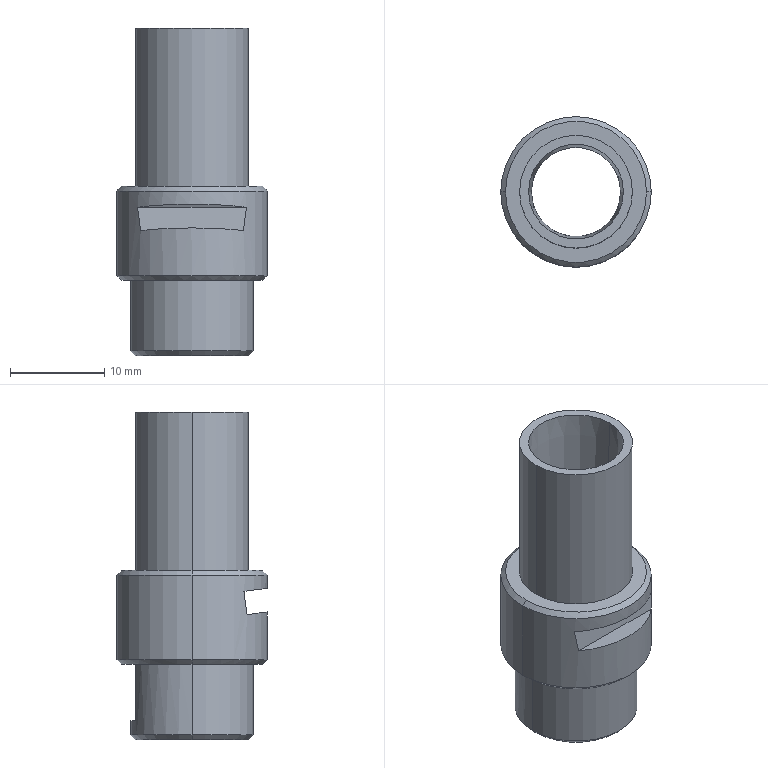Part | SolidWorks | features ICE 4, Chamfer 2, Extrusion 1 | 1 solid | 25 faces | box 16 x 16 x 34.8 mm | volume 2387 mm3 | plane 9 | cone 8 | cylinder 8 | commonest cylinder face diameters 9.5 x2 12 x2 13 x2 16 x2
STEP:
#1=CARTESIAN_POINT('',(7.5,0.,0.));
#2=VERTEX_POINT('',#1);
#3=CARTESIAN_POINT('',(-7.5,0.,0.));
#4=VERTEX_POINT('',#3);
#5=CARTESIAN_POINT('',(0.,0.,0.));
#6=DIRECTION('',(0.,0.,1.));
#7=DIRECTION('',(-1.,0.,0.));
#8=AXIS2_PLACEMENT_3D('',#5,#6,#7);
#9=CIRCLE('',#8,7.5);
#10=EDGE_CURVE('',#2,#4,#9,.T.);
#11=ORIENTED_EDGE('',*,*,#10,.F.);
#12=CARTESIAN_POINT('',(8.,0.,-0.5));
#13=VERTEX_POINT('',#12);
#14=CARTESIAN_POINT('',(8.,0.,-0.5));
#15=DIRECTION('',(0.7071,0.,-0.7071));
#16=VECTOR('',#15,1000.);
#17=LINE('',#14,#16);
#18=EDGE_CURVE('',#2,#13,#17,.T.);
#19=ORIENTED_EDGE('',*,*,#18,.T.);
#20=CARTESIAN_POINT('',(-8.,0.,-0.5));
#21=VERTEX_POINT('',#20);
#22=CARTESIAN_POINT('',(0.,0.,-0.5));
#23=DIRECTION('',(0.,0.,-1.));
#24=DIRECTION('',(-1.,0.,0.));
#25=AXIS2_PLACEMENT_3D('',#22,#23,#24);
#26=CIRCLE('',#25,8.);
#27=EDGE_CURVE('',#21,#13,#26,.T.);
#28=ORIENTED_EDGE('',*,*,#27,.F.);
#29=CARTESIAN_POINT('',(-8.,0.,-0.5));
#30=DIRECTION('',(-0.7071,0.,-0.7071));
#31=VECTOR('',#30,1000.);
#32=LINE('',#29,#31);
#33=EDGE_CURVE('',#4,#21,#32,.T.);
#34=ORIENTED_EDGE('',*,*,#33,.F.);
#35=EDGE_LOOP('',(#11,#19,#28,#34));
#36=FACE_OUTER_BOUND('',#35,.T.);
#37=CARTESIAN_POINT('',(0.,0.,-0.5));
#38=DIRECTION('',(0.,0.,-1.));
#39=DIRECTION('',(-1.,0.,0.));
#40=AXIS2_PLACEMENT_3D('',#37,#38,#39);
#41=CONICAL_SURFACE('',#40,8.,0.7854);
#42=ADVANCED_FACE('',(#36),#41,.T.);
#43=CARTESIAN_POINT('',(-7.5,0.,-10.));
#44=VERTEX_POINT('',#43);
#45=CARTESIAN_POINT('',(7.5,0.,-10.));
#46=VERTEX_POINT('',#45);
#47=CARTESIAN_POINT('',(0.,0.,-10.));
#48=DIRECTION('',(0.,0.,-1.));
#49=DIRECTION('',(-1.,0.,0.));
#50=AXIS2_PLACEMENT_3D('',#47,#48,#49);
#51=CIRCLE('',#50,7.5);
#52=EDGE_CURVE('',#44,#46,#51,.T.);
#53=ORIENTED_EDGE('',*,*,#52,.F.);
#54=CARTESIAN_POINT('',(-8.,0.,-9.5));
#55=VERTEX_POINT('',#54);
#56=CARTESIAN_POINT('',(-7.5,0.,-10.));
#57=DIRECTION('',(-0.7071,0.,0.7071));
#58=VECTOR('',#57,1000.);
#59=LINE('',#56,#58);
#60=EDGE_CURVE('',#44,#55,#59,.T.);
#61=ORIENTED_EDGE('',*,*,#60,.T.);
#62=CARTESIAN_POINT('',(8.,0.,-9.5));
#63=VERTEX_POINT('',#62);
#64=CARTESIAN_POINT('',(0.,0.,-9.5));
#65=DIRECTION('',(0.,0.,1.));
#66=DIRECTION('',(-1.,0.,0.));
#67=AXIS2_PLACEMENT_3D('',#64,#65,#66);
#68=CIRCLE('',#67,8.);
#69=EDGE_CURVE('',#63,#55,#68,.T.);
#70=ORIENTED_EDGE('',*,*,#69,.F.);
#71=CARTESIAN_POINT('',(7.5,0.,-10.));
#72=DIRECTION('',(0.7071,0.,0.7071));
#73=VECTOR('',#72,1000.);
#74=LINE('',#71,#73);
#75=EDGE_CURVE('',#46,#63,#74,.T.);
#76=ORIENTED_EDGE('',*,*,#75,.F.);
#77=EDGE_LOOP('',(#53,#61,#70,#76));
#78=FACE_OUTER_BOUND('',#77,.T.);
#79=CARTESIAN_POINT('',(0.,0.,-10.));
#80=DIRECTION('',(0.,0.,1.));
#81=DIRECTION('',(1.,0.,0.));
#82=AXIS2_PLACEMENT_3D('',#79,#80,#81);
#83=CONICAL_SURFACE('',#82,7.5,0.7854);
#84=ADVANCED_FACE('',(#78),#83,.T.);
#85=CARTESIAN_POINT('',(-6.,0.,-18.));
#86=VERTEX_POINT('',#85);
#87=CARTESIAN_POINT('',(6.,0.,-18.));
#88=VERTEX_POINT('',#87);
#89=CARTESIAN_POINT('',(0.,0.,-18.));
#90=DIRECTION('',(0.,0.,-1.));
#91=DIRECTION('',(-1.,0.,0.));
#92=AXIS2_PLACEMENT_3D('',#89,#90,#91);
#93=CIRCLE('',#92,6.);
#94=EDGE_CURVE('',#86,#88,#93,.T.);
#95=ORIENTED_EDGE('',*,*,#94,.F.);
#96=CARTESIAN_POINT('',(-6.5,0.,-17.5));
#97=VERTEX_POINT('',#96);
#98=CARTESIAN_POINT('',(-6.,0.,-18.));
#99=DIRECTION('',(-0.7071,0.,0.7071));
#100=VECTOR('',#99,1000.);
#101=LINE('',#98,#100);
#102=EDGE_CURVE('',#86,#97,#101,.T.);
#103=ORIENTED_EDGE('',*,*,#102,.T.);
#104=CARTESIAN_POINT('',(6.5,0.,-17.5));
#105=VERTEX_POINT('',#104);
#106=CARTESIAN_POINT('',(0.,0.,-17.5));
#107=DIRECTION('',(0.,0.,1.));
#108=DIRECTION('',(-1.,0.,0.));
#109=AXIS2_PLACEMENT_3D('',#106,#107,#108);
#110=CIRCLE('',#109,6.5);
#111=EDGE_CURVE('',#105,#97,#110,.T.);
#112=ORIENTED_EDGE('',*,*,#111,.F.);
#113=CARTESIAN_POINT('',(6.,0.,-18.));
#114=DIRECTION('',(0.7071,0.,0.7071));
#115=VECTOR('',#114,1000.);
#116=LINE('',#113,#115);
#117=EDGE_CURVE('',#88,#105,#116,.T.);
#118=ORIENTED_EDGE('',*,*,#117,.F.);
#119=EDGE_LOOP('',(#95,#103,#112,#118));
#120=FACE_OUTER_BOUND('',#119,.T.);
#121=CARTESIAN_POINT('',(0.,0.,-18.));
#122=DIRECTION('',(0.,0.,1.));
#123=DIRECTION('',(1.,0.,0.));
#124=AXIS2_PLACEMENT_3D('',#121,#122,#123);
#125=CONICAL_SURFACE('',#124,6.,0.7854);
#126=ADVANCED_FACE('',(#120),#125,.T.);
#127=CARTESIAN_POINT('',(-4.75,0.,6.8));
#128=VERTEX_POINT('',#127);
#129=CARTESIAN_POINT('',(4.75,0.,6.8));
#130=VERTEX_POINT('',#129);
#131=CARTESIAN_POINT('',(0.,0.,6.8));
#132=DIRECTION('',(0.,0.,1.));
#133=DIRECTION('',(1.,0.,0.));
#134=AXIS2_PLACEMENT_3D('',#131,#132,#133);
#135=CIRCLE('',#134,4.75);
#136=EDGE_CURVE('',#128,#130,#135,.T.);
#137=ORIENTED_EDGE('',*,*,#136,.F.);
#138=CARTESIAN_POINT('',(-5.05,0.,16.8));
#139=VERTEX_POINT('',#138);
#140=CARTESIAN_POINT('',(-4.75,0.,6.8));
#141=DIRECTION('',(-0.02999,0.,0.9996));
#142=VECTOR('',#141,1000.);
#143=LINE('',#140,#142);
#144=EDGE_CURVE('',#128,#139,#143,.T.);
#145=ORIENTED_EDGE('',*,*,#144,.T.);
#146=CARTESIAN_POINT('',(5.05,0.,16.8));
#147=VERTEX_POINT('',#146);
#148=CARTESIAN_POINT('',(0.,0.,16.8));
#149=DIRECTION('',(0.,0.,-1.));
#150=DIRECTION('',(1.,0.,0.));
#151=AXIS2_PLACEMENT_3D('',#148,#149,#150);
#152=CIRCLE('',#151,5.05);
#153=EDGE_CURVE('',#147,#139,#152,.T.);
#154=ORIENTED_EDGE('',*,*,#153,.F.);
#155=CARTESIAN_POINT('',(4.75,0.,6.8));
#156=DIRECTION('',(0.02999,0.,0.9996));
#157=VECTOR('',#156,1000.);
#158=LINE('',#155,#157);
#159=EDGE_CURVE('',#130,#147,#158,.T.);
#160=ORIENTED_EDGE('',*,*,#159,.F.);
#161=EDGE_LOOP('',(#137,#145,#154,#160));
#162=FACE_OUTER_BOUND('',#161,.T.);
#163=CARTESIAN_POINT('',(0.,0.,6.8));
#164=DIRECTION('',(0.,0.,1.));
#165=DIRECTION('',(1.,0.,0.));
#166=AXIS2_PLACEMENT_3D('',#163,#164,#165);
#167=CONICAL_SURFACE('',#166,4.75,0.02999);
#168=ADVANCED_FACE('',(#162),#167,.F.);
#169=ORIENTED_EDGE('',*,*,#69,.T.);
#170=CARTESIAN_POINT('',(-8.,0.,-10.));
#171=DIRECTION('',(0.,0.,1.));
#172=VECTOR('',#171,1000.);
#173=LINE('',#170,#172);
#174=EDGE_CURVE('',#55,#21,#173,.T.);
#175=ORIENTED_EDGE('',*,*,#174,.T.);
#176=ORIENTED_EDGE('',*,*,#27,.T.);
#177=CARTESIAN_POINT('',(8.,0.,-10.));
#178=DIRECTION('',(0.,0.,1.));
#179=VECTOR('',#178,1000.);
#180=LINE('',#177,#179);
#181=EDGE_CURVE('',#63,#13,#180,.T.);
#182=ORIENTED_EDGE('',*,*,#181,.F.);
#183=EDGE_LOOP('',(#169,#175,#176,#182));
#184=FACE_OUTER_BOUND('',#183,.T.);
#185=CARTESIAN_POINT('',(0.,0.,-10.));
#186=DIRECTION('',(0.,0.,1.));
#187=DIRECTION('',(1.,0.,0.));
#188=AXIS2_PLACEMENT_3D('',#185,#186,#187);
#189=CYLINDRICAL_SURFACE('',#188,8.);
#190=ADVANCED_FACE('',(#184),#189,.T.);
#191=ORIENTED_EDGE('',*,*,#136,.T.);
#192=CARTESIAN_POINT('',(4.75,0.,-18.));
#193=VERTEX_POINT('',#192);
#194=CARTESIAN_POINT('',(4.75,0.,16.8));
#195=DIRECTION('',(0.,0.,-1.));
#196=VECTOR('',#195,1000.);
#197=LINE('',#194,#196);
#198=EDGE_CURVE('',#130,#193,#197,.T.);
#199=ORIENTED_EDGE('',*,*,#198,.T.);
#200=CARTESIAN_POINT('',(-4.75,0.,-18.));
#201=VERTEX_POINT('',#200);
#202=CARTESIAN_POINT('',(0.,0.,-18.));
#203=DIRECTION('',(0.,0.,-1.));
#204=DIRECTION('',(-1.,0.,0.));
#205=AXIS2_PLACEMENT_3D('',#202,#203,#204);
#206=CIRCLE('',#205,4.75);
#207=EDGE_CURVE('',#193,#201,#206,.T.);
#208=ORIENTED_EDGE('',*,*,#207,.T.);
#209=CARTESIAN_POINT('',(-4.75,0.,16.8));
#210=DIRECTION('',(0.,0.,-1.));
#211=VECTOR('',#210,1000.);
#212=LINE('',#209,#211);
#213=EDGE_CURVE('',#128,#201,#212,.T.);
#214=ORIENTED_EDGE('',*,*,#213,.F.);
#215=EDGE_LOOP('',(#191,#199,#208,#214));
#216=FACE_OUTER_BOUND('',#215,.T.);
#217=CARTESIAN_POINT('',(0.,0.,16.8));
#218=DIRECTION('',(0.,0.,-1.));
#219=DIRECTION('',(-1.,0.,0.));
#220=AXIS2_PLACEMENT_3D('',#217,#218,#219);
#221=CYLINDRICAL_SURFACE('',#220,4.75);
#222=ADVANCED_FACE('',(#216),#221,.F.);
#223=CARTESIAN_POINT('',(6.,0.,16.8));
#224=VERTEX_POINT('',#223);
#225=CARTESIAN_POINT('',(-6.,0.,16.8));
#226=VERTEX_POINT('',#225);
#227=CARTESIAN_POINT('',(0.,0.,16.8));
#228=DIRECTION('',(0.,0.,1.));
#229=DIRECTION('',(1.,0.,0.));
#230=AXIS2_PLACEMENT_3D('',#227,#228,#229);
#231=CIRCLE('',#230,6.);
#232=EDGE_CURVE('',#224,#226,#231,.T.);
#233=ORIENTED_EDGE('',*,*,#232,.F.);
#234=CARTESIAN_POINT('',(6.,0.,0.));
#235=VERTEX_POINT('',#234);
#236=CARTESIAN_POINT('',(6.,0.,16.8));
#237=DIRECTION('',(0.,0.,-1.));
#238=VECTOR('',#237,1000.);
#239=LINE('',#236,#238);
#240=EDGE_CURVE('',#224,#235,#239,.T.);
#241=ORIENTED_EDGE('',*,*,#240,.T.);
#242=CARTESIAN_POINT('',(-6.,0.,0.));
#243=VERTEX_POINT('',#242);
#244=CARTESIAN_POINT('',(0.,0.,0.));
#245=DIRECTION('',(0.,0.,-1.));
#246=DIRECTION('',(-1.,0.,0.));
#247=AXIS2_PLACEMENT_3D('',#244,#245,#246);
#248=CIRCLE('',#247,6.);
#249=EDGE_CURVE('',#243,#235,#248,.T.);
#250=ORIENTED_EDGE('',*,*,#249,.F.);
#251=CARTESIAN_POINT('',(-6.,0.,16.8));
#252=DIRECTION('',(0.,0.,-1.));
#253=VECTOR('',#252,1000.);
#254=LINE('',#251,#253);
#255=EDGE_CURVE('',#226,#243,#254,.T.);
#256=ORIENTED_EDGE('',*,*,#255,.F.);
#257=EDGE_LOOP('',(#233,#241,#250,#256));
#258=FACE_OUTER_BOUND('',#257,.T.);
#259=CARTESIAN_POINT('',(0.,0.,16.8));
#260=DIRECTION('',(0.,0.,-1.));
#261=DIRECTION('',(-1.,0.,0.));
#262=AXIS2_PLACEMENT_3D('',#259,#260,#261);
#263=CYLINDRICAL_SURFACE('',#262,6.);
#264=ADVANCED_FACE('',(#258),#263,.T.);
#265=ORIENTED_EDGE('',*,*,#111,.T.);
#266=CARTESIAN_POINT('',(-6.5,0.,-10.));
#267=VERTEX_POINT('',#266);
#268=CARTESIAN_POINT('',(-6.5,0.,-18.));
#269=DIRECTION('',(0.,0.,1.));
#270=VECTOR('',#269,1000.);
#271=LINE('',#268,#270);
#272=EDGE_CURVE('',#97,#267,#271,.T.);
#273=ORIENTED_EDGE('',*,*,#272,.T.);
#274=CARTESIAN_POINT('',(-2.5,6.,-10.));
#275=VERTEX_POINT('',#274);
#276=CARTESIAN_POINT('',(0.,0.,-10.));
#277=DIRECTION('',(0.,0.,-1.));
#278=DIRECTION('',(-1.,0.,0.));
#279=AXIS2_PLACEMENT_3D('',#276,#277,#278);
#280=CIRCLE('',#279,6.5);
#281=EDGE_CURVE('',#267,#275,#280,.T.);
#282=ORIENTED_EDGE('',*,*,#281,.T.);
#283=CARTESIAN_POINT('',(-2.5,6.,-16.));
#284=VERTEX_POINT('',#283);
#285=CARTESIAN_POINT('',(-2.5,6.,-16.));
#286=DIRECTION('',(0.,0.,1.));
#287=VECTOR('',#286,1000.);
#288=LINE('',#285,#287);
#289=EDGE_CURVE('',#284,#275,#288,.T.);
#290=ORIENTED_EDGE('',*,*,#289,.F.);
#291=CARTESIAN_POINT('',(2.5,6.,-16.));
#292=VERTEX_POINT('',#291);
#293=CARTESIAN_POINT('',(0.,0.,-16.));
#294=DIRECTION('',(0.,0.,-1.));
#295=DIRECTION('',(-1.,0.,0.));
#296=AXIS2_PLACEMENT_3D('',#293,#294,#295);
#297=CIRCLE('',#296,6.5);
#298=EDGE_CURVE('',#284,#292,#297,.T.);
#299=ORIENTED_EDGE('',*,*,#298,.T.);
#300=CARTESIAN_POINT('',(2.5,6.,-10.));
#301=VERTEX_POINT('',#300);
#302=CARTESIAN_POINT('',(2.5,6.,-16.));
#303=DIRECTION('',(0.,0.,1.));
#304=VECTOR('',#303,1000.);
#305=LINE('',#302,#304);
#306=EDGE_CURVE('',#292,#301,#305,.T.);
#307=ORIENTED_EDGE('',*,*,#306,.T.);
#308=CARTESIAN_POINT('',(6.5,0.,-10.));
#309=VERTEX_POINT('',#308);
#310=CARTESIAN_POINT('',(0.,0.,-10.));
#311=DIRECTION('',(0.,0.,-1.));
#312=DIRECTION('',(-1.,0.,0.));
#313=AXIS2_PLACEMENT_3D('',#310,#311,#312);
#314=CIRCLE('',#313,6.5);
#315=EDGE_CURVE('',#301,#309,#314,.T.);
#316=ORIENTED_EDGE('',*,*,#315,.T.);
#317=CARTESIAN_POINT('',(6.5,0.,-18.));
#318=DIRECTION('',(0.,0.,1.));
#319=VECTOR('',#318,1000.);
#320=LINE('',#317,#319);
#321=EDGE_CURVE('',#105,#309,#320,.T.);
#322=ORIENTED_EDGE('',*,*,#321,.F.);
#323=EDGE_LOOP('',(#265,#273,#282,#290,#299,#307,#316,#322));
#324=FACE_OUTER_BOUND('',#323,.T.);
#325=CARTESIAN_POINT('',(0.,0.,-18.));
#326=DIRECTION('',(0.,0.,1.));
#327=DIRECTION('',(1.,0.,0.));
#328=AXIS2_PLACEMENT_3D('',#325,#326,#327);
#329=CYLINDRICAL_SURFACE('',#328,6.5);
#330=ADVANCED_FACE('',(#324),#329,.T.);
#331=ORIENTED_EDGE('',*,*,#272,.F.);
#332=CARTESIAN_POINT('',(0.,0.,-17.5));
#333=DIRECTION('',(0.,0.,1.));
#334=DIRECTION('',(-1.,0.,0.));
#335=AXIS2_PLACEMENT_3D('',#332,#333,#334);
#336=CIRCLE('',#335,6.5);
#337=EDGE_CURVE('',#97,#105,#336,.T.);
#338=ORIENTED_EDGE('',*,*,#337,.T.);
#339=ORIENTED_EDGE('',*,*,#321,.T.);
#340=CARTESIAN_POINT('',(0.,0.,-10.));
#341=DIRECTION('',(0.,0.,-1.));
#342=DIRECTION('',(-1.,0.,0.));
#343=AXIS2_PLACEMENT_3D('',#340,#341,#342);
#344=CIRCLE('',#343,6.5);
#345=EDGE_CURVE('',#309,#267,#344,.T.);
#346=ORIENTED_EDGE('',*,*,#345,.T.);
#347=EDGE_LOOP('',(#331,#338,#339,#346));
#348=FACE_OUTER_BOUND('',#347,.T.);
#349=CARTESIAN_POINT('',(0.,0.,-18.));
#350=DIRECTION('',(0.,0.,1.));
#351=DIRECTION('',(1.,0.,0.));
#352=AXIS2_PLACEMENT_3D('',#349,#350,#351);
#353=CYLINDRICAL_SURFACE('',#352,6.5);
#354=ADVANCED_FACE('',(#348),#353,.T.);
#355=CARTESIAN_POINT('',(0.,0.,-10.));
#356=DIRECTION('',(0.,0.,-1.));
#357=DIRECTION('',(-1.,0.,0.));
#358=AXIS2_PLACEMENT_3D('',#355,#356,#357);
#359=CIRCLE('',#358,7.5);
#360=EDGE_CURVE('',#46,#44,#359,.T.);
#361=ORIENTED_EDGE('',*,*,#360,.T.);
#362=ORIENTED_EDGE('',*,*,#52,.T.);
#363=EDGE_LOOP('',(#361,#362));
#364=FACE_OUTER_BOUND('',#363,.T.);
#365=ORIENTED_EDGE('',*,*,#315,.F.);
#366=CARTESIAN_POINT('',(2.5,6.,-10.));
#367=DIRECTION('',(-1.,0.,0.));
#368=VECTOR('',#367,1000.);
#369=LINE('',#366,#368);
#370=EDGE_CURVE('',#301,#275,#369,.T.);
#371=ORIENTED_EDGE('',*,*,#370,.T.);
#372=ORIENTED_EDGE('',*,*,#281,.F.);
#373=ORIENTED_EDGE('',*,*,#345,.F.);
#374=EDGE_LOOP('',(#365,#371,#372,#373));
#375=FACE_BOUND('',#374,.T.);
#376=CARTESIAN_POINT('',(0.,0.,-10.));
#377=DIRECTION('',(0.,0.,-1.));
#378=DIRECTION('',(-1.,0.,0.));
#379=AXIS2_PLACEMENT_3D('',#376,#377,#378);
#380=PLANE('',#379);
#381=ADVANCED_FACE('',(#364,#375),#380,.T.);
#382=ORIENTED_EDGE('',*,*,#153,.T.);
#383=CARTESIAN_POINT('',(0.,0.,16.8));
#384=DIRECTION('',(0.,0.,-1.));
#385=DIRECTION('',(1.,0.,0.));
#386=AXIS2_PLACEMENT_3D('',#383,#384,#385);
#387=CIRCLE('',#386,5.05);
#388=EDGE_CURVE('',#139,#147,#387,.T.);
#389=ORIENTED_EDGE('',*,*,#388,.T.);
#390=EDGE_LOOP('',(#382,#389));
#391=FACE_BOUND('',#390,.T.);
#392=CARTESIAN_POINT('',(0.,0.,16.8));
#393=DIRECTION('',(0.,0.,1.));
#394=DIRECTION('',(1.,0.,0.));
#395=AXIS2_PLACEMENT_3D('',#392,#393,#394);
#396=CIRCLE('',#395,6.);
#397=EDGE_CURVE('',#226,#224,#396,.T.);
#398=ORIENTED_EDGE('',*,*,#397,.T.);
#399=ORIENTED_EDGE('',*,*,#232,.T.);
#400=EDGE_LOOP('',(#398,#399));
#401=FACE_OUTER_BOUND('',#400,.T.);
#402=CARTESIAN_POINT('',(0.,0.,16.8));
#403=DIRECTION('',(0.,0.,1.));
#404=DIRECTION('',(1.,0.,0.));
#405=AXIS2_PLACEMENT_3D('',#402,#403,#404);
#406=PLANE('',#405);
#407=ADVANCED_FACE('',(#391,#401),#406,.T.);
#408=ORIENTED_EDGE('',*,*,#240,.F.);
#409=ORIENTED_EDGE('',*,*,#397,.F.);
#410=ORIENTED_EDGE('',*,*,#255,.T.);
#411=CARTESIAN_POINT('',(0.,0.,0.));
#412=DIRECTION('',(0.,0.,-1.));
#413=DIRECTION('',(-1.,0.,0.));
#414=AXIS2_PLACEMENT_3D('',#411,#412,#413);
#415=CIRCLE('',#414,6.);
#416=EDGE_CURVE('',#235,#243,#415,.T.);
#417=ORIENTED_EDGE('',*,*,#416,.F.);
#418=EDGE_LOOP('',(#408,#409,#410,#417));
#419=FACE_OUTER_BOUND('',#418,.T.);
#420=CARTESIAN_POINT('',(0.,0.,16.8));
#421=DIRECTION('',(0.,0.,-1.));
#422=DIRECTION('',(-1.,0.,0.));
#423=AXIS2_PLACEMENT_3D('',#420,#421,#422);
#424=CYLINDRICAL_SURFACE('',#423,6.);
#425=ADVANCED_FACE('',(#419),#424,.T.);
#426=ORIENTED_EDGE('',*,*,#198,.F.);
#427=CARTESIAN_POINT('',(0.,0.,6.8));
#428=DIRECTION('',(0.,0.,1.));
#429=DIRECTION('',(1.,0.,0.));
#430=AXIS2_PLACEMENT_3D('',#427,#428,#429);
#431=CIRCLE('',#430,4.75);
#432=EDGE_CURVE('',#130,#128,#431,.T.);
#433=ORIENTED_EDGE('',*,*,#432,.T.);
#434=ORIENTED_EDGE('',*,*,#213,.T.);
#435=CARTESIAN_POINT('',(0.,0.,-18.));
#436=DIRECTION('',(0.,0.,-1.));
#437=DIRECTION('',(-1.,0.,0.));
#438=AXIS2_PLACEMENT_3D('',#435,#436,#437);
#439=CIRCLE('',#438,4.75);
#440=EDGE_CURVE('',#201,#193,#439,.T.);
#441=ORIENTED_EDGE('',*,*,#440,.T.);
#442=EDGE_LOOP('',(#426,#433,#434,#441));
#443=FACE_OUTER_BOUND('',#442,.T.);
#444=CARTESIAN_POINT('',(0.,0.,16.8));
#445=DIRECTION('',(0.,0.,-1.));
#446=DIRECTION('',(-1.,0.,0.));
#447=AXIS2_PLACEMENT_3D('',#444,#445,#446);
#448=CYLINDRICAL_SURFACE('',#447,4.75);
#449=ADVANCED_FACE('',(#443),#448,.F.);
#450=CARTESIAN_POINT('',(0.,0.,0.));
#451=DIRECTION('',(0.,0.,1.));
#452=DIRECTION('',(-1.,0.,0.));
#453=AXIS2_PLACEMENT_3D('',#450,#451,#452);
#454=CIRCLE('',#453,7.5);
#455=EDGE_CURVE('',#4,#2,#454,.T.);
#456=ORIENTED_EDGE('',*,*,#455,.T.);
#457=ORIENTED_EDGE('',*,*,#10,.T.);
#458=EDGE_LOOP('',(#456,#457));
#459=FACE_OUTER_BOUND('',#458,.T.);
#460=ORIENTED_EDGE('',*,*,#249,.T.);
#461=ORIENTED_EDGE('',*,*,#416,.T.);
#462=EDGE_LOOP('',(#460,#461));
#463=FACE_BOUND('',#462,.T.);
#464=CARTESIAN_POINT('',(0.,0.,0.));
#465=DIRECTION('',(0.,0.,-1.));
#466=DIRECTION('',(-1.,0.,0.));
#467=AXIS2_PLACEMENT_3D('',#464,#465,#466);
#468=PLANE('',#467);
#469=ADVANCED_FACE('',(#459,#463),#468,.F.);
#470=ORIENTED_EDGE('',*,*,#174,.F.);
#471=CARTESIAN_POINT('',(0.,0.,-9.5));
#472=DIRECTION('',(0.,0.,1.));
#473=DIRECTION('',(-1.,0.,0.));
#474=AXIS2_PLACEMENT_3D('',#471,#472,#473);
#475=CIRCLE('',#474,8.);
#476=EDGE_CURVE('',#55,#63,#475,.T.);
#477=ORIENTED_EDGE('',*,*,#476,.T.);
#478=ORIENTED_EDGE('',*,*,#181,.T.);
#479=CARTESIAN_POINT('',(0.,0.,-0.5));
#480=DIRECTION('',(0.,0.,-1.));
#481=DIRECTION('',(-1.,0.,0.));
#482=AXIS2_PLACEMENT_3D('',#479,#480,#481);
#483=CIRCLE('',#482,8.);
#484=EDGE_CURVE('',#13,#21,#483,.T.);
#485=ORIENTED_EDGE('',*,*,#484,.T.);
#486=EDGE_LOOP('',(#470,#477,#478,#485));
#487=FACE_OUTER_BOUND('',#486,.T.);
#488=CARTESIAN_POINT('',(-5.789,-5.521,-2.226));
#489=VERTEX_POINT('',#488);
#490=CARTESIAN_POINT('',(5.789,-5.521,-2.226));
#491=VERTEX_POINT('',#490);
#492=CARTESIAN_POINT('',(-5.789,-5.521,-2.226));
#493=CARTESIAN_POINT('',(-2.432,-9.041,-1.763));
#494=CARTESIAN_POINT('',(2.432,-9.041,-1.763));
#495=CARTESIAN_POINT('',(5.789,-5.521,-2.226));
#496=(BOUNDED_CURVE()B_SPLINE_CURVE(3,(#492,#493,#494,#495),.UNSPECIFIED.,.F.,.F.)B_SPLINE_CURVE_WITH_KNOTS((4,4),(5.474,7.092),.UNSPECIFIED.)CURVE()GEOMETRIC_REPRESENTATION_ITEM()RATIONAL_B_SPLINE_CURVE((1.,0.7934,0.7934,1.))REPRESENTATION_ITEM(''));
#497=EDGE_CURVE('',#489,#491,#496,.T.);
#498=ORIENTED_EDGE('',*,*,#497,.T.);
#499=CARTESIAN_POINT('',(5.459,-5.848,-4.705));
#500=VERTEX_POINT('',#499);
#501=CARTESIAN_POINT('',(5.789,-5.521,-2.226));
#502=CARTESIAN_POINT('',(5.682,-5.633,-3.077));
#503=CARTESIAN_POINT('',(5.572,-5.742,-3.903));
#504=CARTESIAN_POINT('',(5.459,-5.848,-4.705));
#505=(BOUNDED_CURVE()B_SPLINE_CURVE(3,(#501,#502,#503,#504),.UNSPECIFIED.,.F.,.F.)B_SPLINE_CURVE_WITH_KNOTS((4,4),(2.333,2.391),.UNSPECIFIED.)CURVE()GEOMETRIC_REPRESENTATION_ITEM()RATIONAL_B_SPLINE_CURVE((1.,0.9997,0.9997,1.))REPRESENTATION_ITEM(''));
#506=EDGE_CURVE('',#491,#500,#505,.T.);
#507=ORIENTED_EDGE('',*,*,#506,.T.);
#508=CARTESIAN_POINT('',(-5.459,-5.848,-4.705));
#509=VERTEX_POINT('',#508);
#510=CARTESIAN_POINT('',(5.459,-5.848,-4.705));
#511=CARTESIAN_POINT('',(2.218,-8.874,-4.306));
#512=CARTESIAN_POINT('',(-2.218,-8.874,-4.306));
#513=CARTESIAN_POINT('',(-5.459,-5.848,-4.705));
#514=(BOUNDED_CURVE()B_SPLINE_CURVE(3,(#510,#511,#512,#513),.UNSPECIFIED.,.F.,.F.)B_SPLINE_CURVE_WITH_KNOTS((4,4),(5.532,7.034),.UNSPECIFIED.)CURVE()GEOMETRIC_REPRESENTATION_ITEM()RATIONAL_B_SPLINE_CURVE((1.,0.8206,0.8206,1.))REPRESENTATION_ITEM(''));
#515=EDGE_CURVE('',#500,#509,#514,.T.);
#516=ORIENTED_EDGE('',*,*,#515,.T.);
#517=CARTESIAN_POINT('',(-5.459,-5.848,-4.705));
#518=CARTESIAN_POINT('',(-5.572,-5.742,-3.903));
#519=CARTESIAN_POINT('',(-5.682,-5.633,-3.077));
#520=CARTESIAN_POINT('',(-5.789,-5.521,-2.226));
#521=(BOUNDED_CURVE()B_SPLINE_CURVE(3,(#517,#518,#519,#520),.UNSPECIFIED.,.F.,.F.)B_SPLINE_CURVE_WITH_KNOTS((4,4),(3.893,3.951),.UNSPECIFIED.)CURVE()GEOMETRIC_REPRESENTATION_ITEM()RATIONAL_B_SPLINE_CURVE((1.,0.9997,0.9997,1.))REPRESENTATION_ITEM(''));
#522=EDGE_CURVE('',#509,#489,#521,.T.);
#523=ORIENTED_EDGE('',*,*,#522,.T.);
#524=EDGE_LOOP('',(#498,#507,#516,#523));
#525=FACE_BOUND('',#524,.T.);
#526=CARTESIAN_POINT('',(0.,0.,-10.));
#527=DIRECTION('',(0.,0.,1.));
#528=DIRECTION('',(1.,0.,0.));
#529=AXIS2_PLACEMENT_3D('',#526,#527,#528);
#530=CYLINDRICAL_SURFACE('',#529,8.);
#531=ADVANCED_FACE('',(#487,#525),#530,.T.);
#532=CARTESIAN_POINT('',(0.,0.,-18.));
#533=DIRECTION('',(0.,0.,-1.));
#534=DIRECTION('',(-1.,0.,0.));
#535=AXIS2_PLACEMENT_3D('',#532,#533,#534);
#536=CIRCLE('',#535,6.);
#537=EDGE_CURVE('',#88,#86,#536,.T.);
#538=ORIENTED_EDGE('',*,*,#537,.T.);
#539=ORIENTED_EDGE('',*,*,#94,.T.);
#540=EDGE_LOOP('',(#538,#539));
#541=FACE_OUTER_BOUND('',#540,.T.);
#542=ORIENTED_EDGE('',*,*,#440,.F.);
#543=ORIENTED_EDGE('',*,*,#207,.F.);
#544=EDGE_LOOP('',(#542,#543));
#545=FACE_BOUND('',#544,.T.);
#546=CARTESIAN_POINT('',(0.,0.,-18.));
#547=DIRECTION('',(0.,0.,-1.));
#548=DIRECTION('',(-1.,0.,0.));
#549=AXIS2_PLACEMENT_3D('',#546,#547,#548);
#550=PLANE('',#549);
#551=ADVANCED_FACE('',(#541,#545),#550,.T.);
#552=ORIENTED_EDGE('',*,*,#144,.F.);
#553=ORIENTED_EDGE('',*,*,#432,.F.);
#554=ORIENTED_EDGE('',*,*,#159,.T.);
#555=ORIENTED_EDGE('',*,*,#388,.F.);
#556=EDGE_LOOP('',(#552,#553,#554,#555));
#557=FACE_OUTER_BOUND('',#556,.T.);
#558=CARTESIAN_POINT('',(0.,0.,6.8));
#559=DIRECTION('',(0.,0.,1.));
#560=DIRECTION('',(1.,0.,0.));
#561=AXIS2_PLACEMENT_3D('',#558,#559,#560);
#562=CONICAL_SURFACE('',#561,4.75,0.02999);
#563=ADVANCED_FACE('',(#557),#562,.F.);
#564=ORIENTED_EDGE('',*,*,#497,.F.);
#565=CARTESIAN_POINT('',(-8.,-5.521,-2.226));
#566=DIRECTION('',(1.,0.,0.));
#567=VECTOR('',#566,1000.);
#568=LINE('',#565,#567);
#569=EDGE_CURVE('',#489,#491,#568,.T.);
#570=ORIENTED_EDGE('',*,*,#569,.T.);
#571=EDGE_LOOP('',(#564,#570));
#572=FACE_OUTER_BOUND('',#571,.T.);
#573=CARTESIAN_POINT('',(-8.,-8.,-1.9));
#574=DIRECTION('',(0.,0.1305,0.9914));
#575=DIRECTION('',(0.,-0.9914,0.1305));
#576=AXIS2_PLACEMENT_3D('',#573,#574,#575);
#577=PLANE('',#576);
#578=ADVANCED_FACE('',(#572),#577,.F.);
#579=ORIENTED_EDGE('',*,*,#569,.F.);
#580=ORIENTED_EDGE('',*,*,#522,.F.);
#581=CARTESIAN_POINT('',(-8.,-5.848,-4.705));
#582=DIRECTION('',(1.,0.,0.));
#583=VECTOR('',#582,1000.);
#584=LINE('',#581,#583);
#585=EDGE_CURVE('',#509,#500,#584,.T.);
#586=ORIENTED_EDGE('',*,*,#585,.T.);
#587=ORIENTED_EDGE('',*,*,#506,.F.);
#588=EDGE_LOOP('',(#579,#580,#586,#587));
#589=FACE_OUTER_BOUND('',#588,.T.);
#590=CARTESIAN_POINT('',(-8.,-5.521,-2.226));
#591=DIRECTION('',(0.,0.9914,-0.1305));
#592=DIRECTION('',(0.,0.1305,0.9914));
#593=AXIS2_PLACEMENT_3D('',#590,#591,#592);
#594=PLANE('',#593);
#595=ADVANCED_FACE('',(#589),#594,.F.);
#596=ORIENTED_EDGE('',*,*,#515,.F.);
#597=ORIENTED_EDGE('',*,*,#585,.F.);
#598=EDGE_LOOP('',(#596,#597));
#599=FACE_OUTER_BOUND('',#598,.T.);
#600=CARTESIAN_POINT('',(-8.,-5.848,-4.705));
#601=DIRECTION('',(0.,-0.1305,-0.9914));
#602=DIRECTION('',(0.,0.9914,-0.1305));
#603=AXIS2_PLACEMENT_3D('',#600,#601,#602);
#604=PLANE('',#603);
#605=ADVANCED_FACE('',(#599),#604,.F.);
#606=ORIENTED_EDGE('',*,*,#370,.F.);
#607=ORIENTED_EDGE('',*,*,#306,.F.);
#608=CARTESIAN_POINT('',(2.5,6.,-16.));
#609=DIRECTION('',(-1.,0.,0.));
#610=VECTOR('',#609,1000.);
#611=LINE('',#608,#610);
#612=EDGE_CURVE('',#292,#284,#611,.T.);
#613=ORIENTED_EDGE('',*,*,#612,.T.);
#614=ORIENTED_EDGE('',*,*,#289,.T.);
#615=EDGE_LOOP('',(#606,#607,#613,#614));
#616=FACE_OUTER_BOUND('',#615,.T.);
#617=CARTESIAN_POINT('',(2.5,6.,-16.));
#618=DIRECTION('',(0.,1.,0.));
#619=DIRECTION('',(0.,0.,1.));
#620=AXIS2_PLACEMENT_3D('',#617,#618,#619);
#621=PLANE('',#620);
#622=ADVANCED_FACE('',(#616),#621,.T.);
#623=ORIENTED_EDGE('',*,*,#298,.F.);
#624=ORIENTED_EDGE('',*,*,#612,.F.);
#625=EDGE_LOOP('',(#623,#624));
#626=FACE_OUTER_BOUND('',#625,.T.);
#627=CARTESIAN_POINT('',(0.,0.,-16.));
#628=DIRECTION('',(0.,0.,-1.));
#629=DIRECTION('',(-1.,0.,0.));
#630=AXIS2_PLACEMENT_3D('',#627,#628,#629);
#631=PLANE('',#630);
#632=ADVANCED_FACE('',(#626),#631,.F.);
#633=ORIENTED_EDGE('',*,*,#102,.F.);
#634=ORIENTED_EDGE('',*,*,#537,.F.);
#635=ORIENTED_EDGE('',*,*,#117,.T.);
#636=ORIENTED_EDGE('',*,*,#337,.F.);
#637=EDGE_LOOP('',(#633,#634,#635,#636));
#638=FACE_OUTER_BOUND('',#637,.T.);
#639=CARTESIAN_POINT('',(0.,0.,-18.));
#640=DIRECTION('',(0.,0.,1.));
#641=DIRECTION('',(1.,0.,0.));
#642=AXIS2_PLACEMENT_3D('',#639,#640,#641);
#643=CONICAL_SURFACE('',#642,6.,0.7854);
#644=ADVANCED_FACE('',(#638),#643,.T.);
#645=ORIENTED_EDGE('',*,*,#60,.F.);
#646=ORIENTED_EDGE('',*,*,#360,.F.);
#647=ORIENTED_EDGE('',*,*,#75,.T.);
#648=ORIENTED_EDGE('',*,*,#476,.F.);
#649=EDGE_LOOP('',(#645,#646,#647,#648));
#650=FACE_OUTER_BOUND('',#649,.T.);
#651=CARTESIAN_POINT('',(0.,0.,-10.));
#652=DIRECTION('',(0.,0.,1.));
#653=DIRECTION('',(1.,0.,0.));
#654=AXIS2_PLACEMENT_3D('',#651,#652,#653);
#655=CONICAL_SURFACE('',#654,7.5,0.7854);
#656=ADVANCED_FACE('',(#650),#655,.T.);
#657=ORIENTED_EDGE('',*,*,#18,.F.);
#658=ORIENTED_EDGE('',*,*,#455,.F.);
#659=ORIENTED_EDGE('',*,*,#33,.T.);
#660=ORIENTED_EDGE('',*,*,#484,.F.);
#661=EDGE_LOOP('',(#657,#658,#659,#660));
#662=FACE_OUTER_BOUND('',#661,.T.);
#663=CARTESIAN_POINT('',(0.,0.,-0.5));
#664=DIRECTION('',(0.,0.,-1.));
#665=DIRECTION('',(-1.,0.,0.));
#666=AXIS2_PLACEMENT_3D('',#663,#664,#665);
#667=CONICAL_SURFACE('',#666,8.,0.7854);
#668=ADVANCED_FACE('',(#662),#667,.T.);
#669=CLOSED_SHELL('',(#42,#84,#126,#168,#190,#222,#264,#330,#354,#381,#407,#425,#449,#469,#531,#551,#563,#578,#595,#605,#622,#632,#644,#656,#668));
#670=MANIFOLD_SOLID_BREP('',#669);
#671=CARTESIAN_POINT('',(0.,0.,0.));
#672=DIRECTION('',(0.,0.,1.));
#673=DIRECTION('',(1.,0.,0.));
#674=AXIS2_PLACEMENT_3D('',#671,#672,#673);
#675=(LENGTH_UNIT()NAMED_UNIT(*)SI_UNIT(.MILLI.,.METRE.));
#676=UNCERTAINTY_MEASURE_WITH_UNIT(LENGTH_MEASURE(0.00001),#675,'','');
#677=(NAMED_UNIT(*)PLANE_ANGLE_UNIT()SI_UNIT($,.RADIAN.));
#678=(NAMED_UNIT(*)SI_UNIT($,.STERADIAN.)SOLID_ANGLE_UNIT());
#679=(GEOMETRIC_REPRESENTATION_CONTEXT(3)GLOBAL_UNCERTAINTY_ASSIGNED_CONTEXT((#676))GLOBAL_UNIT_ASSIGNED_CONTEXT((#675,#677,#678))REPRESENTATION_CONTEXT('',''));
#680=ADVANCED_BREP_SHAPE_REPRESENTATION('',(#670,#674),#679);